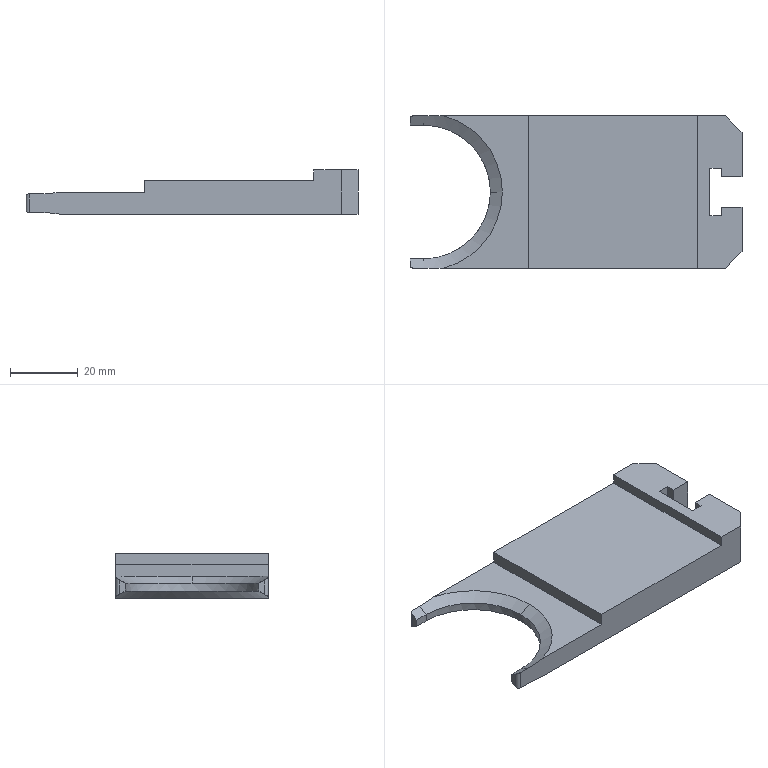Part | SolidWorks | features Chamfer 5, ICE 4, Fillet 2, Cavity 1, Cut 1, Extrusion 1 | 1 solid | 33 faces | box 98 x 45 x 13 mm | volume 33070 mm3 | plane 27 | cone 3 | cylinder 3 | commonest cylinder face diameters 2 x2 39.5 x1
STEP:
#1=CARTESIAN_POINT('',(23.75,0.,-5.62));
#2=VERTEX_POINT('',#1);
#3=CARTESIAN_POINT('',(4.,19.75,-5.62));
#4=VERTEX_POINT('',#3);
#5=CARTESIAN_POINT('',(4.,0.,-5.62));
#6=DIRECTION('',(0.,0.,1.));
#7=DIRECTION('',(-1.,0.,0.));
#8=AXIS2_PLACEMENT_3D('',#5,#6,#7);
#9=CIRCLE('',#8,19.75);
#10=EDGE_CURVE('',#2,#4,#9,.T.);
#11=ORIENTED_EDGE('',*,*,#10,.F.);
#12=CARTESIAN_POINT('',(27.25,0.,-3.6));
#13=VERTEX_POINT('',#12);
#14=CARTESIAN_POINT('',(23.75,0.,-5.62));
#15=DIRECTION('',(0.8661,0.,0.4999));
#16=VECTOR('',#15,1000.);
#17=LINE('',#14,#16);
#18=EDGE_CURVE('',#2,#13,#17,.T.);
#19=ORIENTED_EDGE('',*,*,#18,.T.);
#20=CARTESIAN_POINT('',(9.858,22.5,-3.6));
#21=VERTEX_POINT('',#20);
#22=CARTESIAN_POINT('',(4.,0.,-3.6));
#23=DIRECTION('',(0.,0.,-1.));
#24=DIRECTION('',(-1.,0.,0.));
#25=AXIS2_PLACEMENT_3D('',#22,#23,#24);
#26=CIRCLE('',#25,23.25);
#27=EDGE_CURVE('',#21,#13,#26,.T.);
#28=ORIENTED_EDGE('',*,*,#27,.F.);
#29=CARTESIAN_POINT('',(4.,22.5,-4.033));
#30=VERTEX_POINT('',#29);
#31=CARTESIAN_POINT('',(4.,22.5,-4.033));
#32=CARTESIAN_POINT('',(5.951,22.5,-4.033));
#33=CARTESIAN_POINT('',(7.904,22.5,-3.884));
#34=CARTESIAN_POINT('',(9.858,22.5,-3.6));
#35=B_SPLINE_CURVE_WITH_KNOTS('',3,(#31,#32,#33,#34),.UNSPECIFIED.,.F.,.F.,(4,4),(0.006759,0.01261),.UNSPECIFIED.);
#36=EDGE_CURVE('',#30,#21,#35,.T.);
#37=ORIENTED_EDGE('',*,*,#36,.F.);
#38=CARTESIAN_POINT('',(4.,23.25,-3.6));
#39=DIRECTION('',(0.,-0.8661,-0.4999));
#40=VECTOR('',#39,1000.);
#41=LINE('',#38,#40);
#42=EDGE_CURVE('',#30,#4,#41,.T.);
#43=ORIENTED_EDGE('',*,*,#42,.T.);
#44=EDGE_LOOP('',(#11,#19,#28,#37,#43));
#45=FACE_OUTER_BOUND('',#44,.T.);
#46=CARTESIAN_POINT('',(4.,0.,-5.62));
#47=DIRECTION('',(0.,0.,1.));
#48=DIRECTION('',(1.,0.,0.));
#49=AXIS2_PLACEMENT_3D('',#46,#47,#48);
#50=CONICAL_SURFACE('',#49,19.75,1.047);
#51=ADVANCED_FACE('',(#45),#50,.F.);
#52=CARTESIAN_POINT('',(0.,-21.5,-8.99));
#53=VERTEX_POINT('',#52);
#54=CARTESIAN_POINT('',(0.,-21.5,-4.61));
#55=VERTEX_POINT('',#54);
#56=CARTESIAN_POINT('',(0.,-21.5,-10.));
#57=DIRECTION('',(0.,0.,1.));
#58=VECTOR('',#57,1000.);
#59=LINE('',#56,#58);
#60=EDGE_CURVE('',#53,#55,#59,.T.);
#61=ORIENTED_EDGE('',*,*,#60,.T.);
#62=CARTESIAN_POINT('',(0.,-19.75,-5.62));
#63=VERTEX_POINT('',#62);
#64=CARTESIAN_POINT('',(0.,-19.75,-5.62));
#65=DIRECTION('',(0.,0.8661,-0.4999));
#66=VECTOR('',#65,1000.);
#67=LINE('',#64,#66);
#68=EDGE_CURVE('',#55,#63,#67,.T.);
#69=ORIENTED_EDGE('',*,*,#68,.T.);
#70=CARTESIAN_POINT('',(0.,-19.75,-7.98));
#71=VERTEX_POINT('',#70);
#72=CARTESIAN_POINT('',(0.,-19.75,3.001));
#73=DIRECTION('',(0.,0.,1.));
#74=VECTOR('',#73,1000.);
#75=LINE('',#72,#74);
#76=EDGE_CURVE('',#71,#63,#75,.T.);
#77=ORIENTED_EDGE('',*,*,#76,.F.);
#78=CARTESIAN_POINT('',(0.,-19.75,-7.98));
#79=DIRECTION('',(0.,-0.8661,-0.4999));
#80=VECTOR('',#79,1000.);
#81=LINE('',#78,#80);
#82=EDGE_CURVE('',#71,#53,#81,.T.);
#83=ORIENTED_EDGE('',*,*,#82,.T.);
#84=EDGE_LOOP('',(#61,#69,#77,#83));
#85=FACE_OUTER_BOUND('',#84,.T.);
#86=CARTESIAN_POINT('',(0.,22.5,-10.));
#87=DIRECTION('',(1.,0.,0.));
#88=DIRECTION('',(0.,0.,-1.));
#89=AXIS2_PLACEMENT_3D('',#86,#87,#88);
#90=PLANE('',#89);
#91=ADVANCED_FACE('',(#85),#90,.F.);
#92=CARTESIAN_POINT('',(98.,17.5,3.));
#93=VERTEX_POINT('',#92);
#94=CARTESIAN_POINT('',(98.,4.5,3.));
#95=VERTEX_POINT('',#94);
#96=CARTESIAN_POINT('',(98.,22.5,3.));
#97=DIRECTION('',(0.,-1.,0.));
#98=VECTOR('',#97,1000.);
#99=LINE('',#96,#98);
#100=EDGE_CURVE('',#93,#95,#99,.T.);
#101=ORIENTED_EDGE('',*,*,#100,.T.);
#102=CARTESIAN_POINT('',(98.,4.5,-10.));
#103=VERTEX_POINT('',#102);
#104=CARTESIAN_POINT('',(98.,4.5,3.001));
#105=DIRECTION('',(0.,0.,-1.));
#106=VECTOR('',#105,1000.);
#107=LINE('',#104,#106);
#108=EDGE_CURVE('',#95,#103,#107,.T.);
#109=ORIENTED_EDGE('',*,*,#108,.T.);
#110=CARTESIAN_POINT('',(98.,17.5,-10.));
#111=VERTEX_POINT('',#110);
#112=CARTESIAN_POINT('',(98.,22.5,-10.));
#113=DIRECTION('',(0.,-1.,0.));
#114=VECTOR('',#113,1000.);
#115=LINE('',#112,#114);
#116=EDGE_CURVE('',#111,#103,#115,.T.);
#117=ORIENTED_EDGE('',*,*,#116,.F.);
#118=CARTESIAN_POINT('',(98.,17.5,3.));
#119=DIRECTION('',(0.,0.,1.));
#120=VECTOR('',#119,1000.);
#121=LINE('',#118,#120);
#122=EDGE_CURVE('',#111,#93,#121,.T.);
#123=ORIENTED_EDGE('',*,*,#122,.T.);
#124=EDGE_LOOP('',(#101,#109,#117,#123));
#125=FACE_OUTER_BOUND('',#124,.T.);
#126=CARTESIAN_POINT('',(98.,22.5,3.));
#127=DIRECTION('',(-1.,0.,0.));
#128=DIRECTION('',(0.,0.,1.));
#129=AXIS2_PLACEMENT_3D('',#126,#127,#128);
#130=PLANE('',#129);
#131=ADVANCED_FACE('',(#125),#130,.F.);
#132=CARTESIAN_POINT('',(0.,19.75,-5.62));
#133=VERTEX_POINT('',#132);
#134=CARTESIAN_POINT('',(0.,19.75,-7.98));
#135=VERTEX_POINT('',#134);
#136=CARTESIAN_POINT('',(0.,19.75,3.001));
#137=DIRECTION('',(0.,0.,-1.));
#138=VECTOR('',#137,1000.);
#139=LINE('',#136,#138);
#140=EDGE_CURVE('',#133,#135,#139,.T.);
#141=ORIENTED_EDGE('',*,*,#140,.F.);
#142=CARTESIAN_POINT('',(0.,21.5,-4.61));
#143=VERTEX_POINT('',#142);
#144=CARTESIAN_POINT('',(0.,19.75,-5.62));
#145=DIRECTION('',(0.,0.8661,0.4999));
#146=VECTOR('',#145,1000.);
#147=LINE('',#144,#146);
#148=EDGE_CURVE('',#133,#143,#147,.T.);
#149=ORIENTED_EDGE('',*,*,#148,.T.);
#150=CARTESIAN_POINT('',(0.,21.5,-8.99));
#151=VERTEX_POINT('',#150);
#152=CARTESIAN_POINT('',(0.,21.5,-10.));
#153=DIRECTION('',(0.,0.,-1.));
#154=VECTOR('',#153,1000.);
#155=LINE('',#152,#154);
#156=EDGE_CURVE('',#143,#151,#155,.T.);
#157=ORIENTED_EDGE('',*,*,#156,.T.);
#158=CARTESIAN_POINT('',(0.,19.75,-7.98));
#159=DIRECTION('',(0.,-0.8661,0.4999));
#160=VECTOR('',#159,1000.);
#161=LINE('',#158,#160);
#162=EDGE_CURVE('',#151,#135,#161,.T.);
#163=ORIENTED_EDGE('',*,*,#162,.T.);
#164=EDGE_LOOP('',(#141,#149,#157,#163));
#165=FACE_OUTER_BOUND('',#164,.T.);
#166=CARTESIAN_POINT('',(0.,22.5,-10.));
#167=DIRECTION('',(1.,0.,0.));
#168=DIRECTION('',(0.,0.,-1.));
#169=AXIS2_PLACEMENT_3D('',#166,#167,#168);
#170=PLANE('',#169);
#171=ADVANCED_FACE('',(#165),#170,.F.);
#172=CARTESIAN_POINT('',(35.,22.5,0.));
#173=VERTEX_POINT('',#172);
#174=CARTESIAN_POINT('',(85.,22.5,0.));
#175=VERTEX_POINT('',#174);
#176=CARTESIAN_POINT('',(0.,22.5,0.));
#177=DIRECTION('',(1.,0.,0.));
#178=VECTOR('',#177,1000.);
#179=LINE('',#176,#178);
#180=EDGE_CURVE('',#173,#175,#179,.T.);
#181=ORIENTED_EDGE('',*,*,#180,.F.);
#182=CARTESIAN_POINT('',(35.,-22.5,0.));
#183=VERTEX_POINT('',#182);
#184=CARTESIAN_POINT('',(35.,22.5,0.));
#185=DIRECTION('',(0.,-1.,0.));
#186=VECTOR('',#185,1000.);
#187=LINE('',#184,#186);
#188=EDGE_CURVE('',#173,#183,#187,.T.);
#189=ORIENTED_EDGE('',*,*,#188,.T.);
#190=CARTESIAN_POINT('',(85.,-22.5,0.));
#191=VERTEX_POINT('',#190);
#192=CARTESIAN_POINT('',(0.,-22.5,0.));
#193=DIRECTION('',(1.,0.,0.));
#194=VECTOR('',#193,1000.);
#195=LINE('',#192,#194);
#196=EDGE_CURVE('',#183,#191,#195,.T.);
#197=ORIENTED_EDGE('',*,*,#196,.T.);
#198=CARTESIAN_POINT('',(85.,22.5,0.));
#199=DIRECTION('',(0.,-1.,0.));
#200=VECTOR('',#199,1000.);
#201=LINE('',#198,#200);
#202=EDGE_CURVE('',#175,#191,#201,.T.);
#203=ORIENTED_EDGE('',*,*,#202,.F.);
#204=EDGE_LOOP('',(#181,#189,#197,#203));
#205=FACE_OUTER_BOUND('',#204,.T.);
#206=CARTESIAN_POINT('',(0.,22.5,0.));
#207=DIRECTION('',(0.,0.,-1.));
#208=DIRECTION('',(-1.,0.,0.));
#209=AXIS2_PLACEMENT_3D('',#206,#207,#208);
#210=PLANE('',#209);
#211=ADVANCED_FACE('',(#205),#210,.F.);
#212=CARTESIAN_POINT('',(85.,-22.5,3.));
#213=VERTEX_POINT('',#212);
#214=CARTESIAN_POINT('',(85.,-22.5,0.));
#215=DIRECTION('',(0.,0.,1.));
#216=VECTOR('',#215,1000.);
#217=LINE('',#214,#216);
#218=EDGE_CURVE('',#191,#213,#217,.T.);
#219=ORIENTED_EDGE('',*,*,#218,.T.);
#220=CARTESIAN_POINT('',(85.,22.5,3.));
#221=VERTEX_POINT('',#220);
#222=CARTESIAN_POINT('',(85.,22.5,3.));
#223=DIRECTION('',(0.,-1.,0.));
#224=VECTOR('',#223,1000.);
#225=LINE('',#222,#224);
#226=EDGE_CURVE('',#221,#213,#225,.T.);
#227=ORIENTED_EDGE('',*,*,#226,.F.);
#228=CARTESIAN_POINT('',(85.,22.5,0.));
#229=DIRECTION('',(0.,0.,1.));
#230=VECTOR('',#229,1000.);
#231=LINE('',#228,#230);
#232=EDGE_CURVE('',#175,#221,#231,.T.);
#233=ORIENTED_EDGE('',*,*,#232,.F.);
#234=ORIENTED_EDGE('',*,*,#202,.T.);
#235=EDGE_LOOP('',(#219,#227,#233,#234));
#236=FACE_OUTER_BOUND('',#235,.T.);
#237=CARTESIAN_POINT('',(85.,22.5,0.));
#238=DIRECTION('',(1.,0.,0.));
#239=DIRECTION('',(0.,0.,-1.));
#240=AXIS2_PLACEMENT_3D('',#237,#238,#239);
#241=PLANE('',#240);
#242=ADVANCED_FACE('',(#236),#241,.F.);
#243=CARTESIAN_POINT('',(92.,4.5,3.));
#244=VERTEX_POINT('',#243);
#245=CARTESIAN_POINT('',(92.,7.,3.));
#246=VERTEX_POINT('',#245);
#247=CARTESIAN_POINT('',(92.,4.5,3.));
#248=DIRECTION('',(0.,1.,0.));
#249=VECTOR('',#248,1000.);
#250=LINE('',#247,#249);
#251=EDGE_CURVE('',#244,#246,#250,.T.);
#252=ORIENTED_EDGE('',*,*,#251,.F.);
#253=CARTESIAN_POINT('',(98.,4.5,3.));
#254=DIRECTION('',(-1.,0.,0.));
#255=VECTOR('',#254,1000.);
#256=LINE('',#253,#255);
#257=EDGE_CURVE('',#95,#244,#256,.T.);
#258=ORIENTED_EDGE('',*,*,#257,.F.);
#259=ORIENTED_EDGE('',*,*,#100,.F.);
#260=CARTESIAN_POINT('',(93.,22.5,3.));
#261=VERTEX_POINT('',#260);
#262=CARTESIAN_POINT('',(93.,22.5,3.));
#263=DIRECTION('',(-0.7071,0.7071,0.));
#264=VECTOR('',#263,1000.);
#265=LINE('',#262,#264);
#266=EDGE_CURVE('',#93,#261,#265,.T.);
#267=ORIENTED_EDGE('',*,*,#266,.T.);
#268=CARTESIAN_POINT('',(85.,22.5,3.));
#269=DIRECTION('',(1.,0.,0.));
#270=VECTOR('',#269,1000.);
#271=LINE('',#268,#270);
#272=EDGE_CURVE('',#221,#261,#271,.T.);
#273=ORIENTED_EDGE('',*,*,#272,.F.);
#274=ORIENTED_EDGE('',*,*,#226,.T.);
#275=CARTESIAN_POINT('',(93.,-22.5,3.));
#276=VERTEX_POINT('',#275);
#277=CARTESIAN_POINT('',(85.,-22.5,3.));
#278=DIRECTION('',(1.,0.,0.));
#279=VECTOR('',#278,1000.);
#280=LINE('',#277,#279);
#281=EDGE_CURVE('',#213,#276,#280,.T.);
#282=ORIENTED_EDGE('',*,*,#281,.T.);
#283=CARTESIAN_POINT('',(98.,-17.5,3.));
#284=VERTEX_POINT('',#283);
#285=CARTESIAN_POINT('',(98.,-17.5,3.));
#286=DIRECTION('',(0.7071,0.7071,0.));
#287=VECTOR('',#286,1000.);
#288=LINE('',#285,#287);
#289=EDGE_CURVE('',#276,#284,#288,.T.);
#290=ORIENTED_EDGE('',*,*,#289,.T.);
#291=CARTESIAN_POINT('',(98.,-4.5,3.));
#292=VERTEX_POINT('',#291);
#293=CARTESIAN_POINT('',(98.,22.5,3.));
#294=DIRECTION('',(0.,-1.,0.));
#295=VECTOR('',#294,1000.);
#296=LINE('',#293,#295);
#297=EDGE_CURVE('',#292,#284,#296,.T.);
#298=ORIENTED_EDGE('',*,*,#297,.F.);
#299=CARTESIAN_POINT('',(92.,-4.5,3.));
#300=VERTEX_POINT('',#299);
#301=CARTESIAN_POINT('',(92.,-4.5,3.));
#302=DIRECTION('',(1.,0.,0.));
#303=VECTOR('',#302,1000.);
#304=LINE('',#301,#303);
#305=EDGE_CURVE('',#300,#292,#304,.T.);
#306=ORIENTED_EDGE('',*,*,#305,.F.);
#307=CARTESIAN_POINT('',(92.,-7.,3.));
#308=VERTEX_POINT('',#307);
#309=CARTESIAN_POINT('',(92.,-7.,3.));
#310=DIRECTION('',(0.,1.,0.));
#311=VECTOR('',#310,1000.);
#312=LINE('',#309,#311);
#313=EDGE_CURVE('',#308,#300,#312,.T.);
#314=ORIENTED_EDGE('',*,*,#313,.F.);
#315=CARTESIAN_POINT('',(88.5,-7.,3.));
#316=VERTEX_POINT('',#315);
#317=CARTESIAN_POINT('',(88.5,-7.,3.));
#318=DIRECTION('',(1.,0.,0.));
#319=VECTOR('',#318,1000.);
#320=LINE('',#317,#319);
#321=EDGE_CURVE('',#316,#308,#320,.T.);
#322=ORIENTED_EDGE('',*,*,#321,.F.);
#323=CARTESIAN_POINT('',(88.5,7.,3.));
#324=VERTEX_POINT('',#323);
#325=CARTESIAN_POINT('',(88.5,7.,3.));
#326=DIRECTION('',(0.,-1.,0.));
#327=VECTOR('',#326,1000.);
#328=LINE('',#325,#327);
#329=EDGE_CURVE('',#324,#316,#328,.T.);
#330=ORIENTED_EDGE('',*,*,#329,.F.);
#331=CARTESIAN_POINT('',(92.,7.,3.));
#332=DIRECTION('',(-1.,0.,0.));
#333=VECTOR('',#332,1000.);
#334=LINE('',#331,#333);
#335=EDGE_CURVE('',#246,#324,#334,.T.);
#336=ORIENTED_EDGE('',*,*,#335,.F.);
#337=EDGE_LOOP('',(#252,#258,#259,#267,#273,#274,#282,#290,#298,#306,#314,#322,#330,#336));
#338=FACE_OUTER_BOUND('',#337,.T.);
#339=CARTESIAN_POINT('',(85.,22.5,3.));
#340=DIRECTION('',(0.,0.,-1.));
#341=DIRECTION('',(-1.,0.,0.));
#342=AXIS2_PLACEMENT_3D('',#339,#340,#341);
#343=PLANE('',#342);
#344=ADVANCED_FACE('',(#338),#343,.F.);
#345=CARTESIAN_POINT('',(98.,-4.5,-10.));
#346=VERTEX_POINT('',#345);
#347=CARTESIAN_POINT('',(98.,-17.5,-10.));
#348=VERTEX_POINT('',#347);
#349=CARTESIAN_POINT('',(98.,22.5,-10.));
#350=DIRECTION('',(0.,-1.,0.));
#351=VECTOR('',#350,1000.);
#352=LINE('',#349,#351);
#353=EDGE_CURVE('',#346,#348,#352,.T.);
#354=ORIENTED_EDGE('',*,*,#353,.F.);
#355=CARTESIAN_POINT('',(98.,-4.5,3.001));
#356=DIRECTION('',(0.,0.,-1.));
#357=VECTOR('',#356,1000.);
#358=LINE('',#355,#357);
#359=EDGE_CURVE('',#292,#346,#358,.T.);
#360=ORIENTED_EDGE('',*,*,#359,.F.);
#361=ORIENTED_EDGE('',*,*,#297,.T.);
#362=CARTESIAN_POINT('',(98.,-17.5,3.));
#363=DIRECTION('',(0.,0.,-1.));
#364=VECTOR('',#363,1000.);
#365=LINE('',#362,#364);
#366=EDGE_CURVE('',#284,#348,#365,.T.);
#367=ORIENTED_EDGE('',*,*,#366,.T.);
#368=EDGE_LOOP('',(#354,#360,#361,#367));
#369=FACE_OUTER_BOUND('',#368,.T.);
#370=CARTESIAN_POINT('',(98.,22.5,3.));
#371=DIRECTION('',(-1.,0.,0.));
#372=DIRECTION('',(0.,0.,1.));
#373=AXIS2_PLACEMENT_3D('',#370,#371,#372);
#374=PLANE('',#373);
#375=ADVANCED_FACE('',(#369),#374,.F.);
#376=CARTESIAN_POINT('',(93.,-22.5,-10.));
#377=VERTEX_POINT('',#376);
#378=CARTESIAN_POINT('',(9.858,-22.5,-10.));
#379=VERTEX_POINT('',#378);
#380=CARTESIAN_POINT('',(98.,-22.5,-10.));
#381=DIRECTION('',(-1.,0.,0.));
#382=VECTOR('',#381,1000.);
#383=LINE('',#380,#382);
#384=EDGE_CURVE('',#377,#379,#383,.T.);
#385=ORIENTED_EDGE('',*,*,#384,.T.);
#386=CARTESIAN_POINT('',(9.858,22.5,-10.));
#387=VERTEX_POINT('',#386);
#388=CARTESIAN_POINT('',(4.,0.,-10.));
#389=DIRECTION('',(0.,0.,1.));
#390=DIRECTION('',(1.,0.,0.));
#391=AXIS2_PLACEMENT_3D('',#388,#389,#390);
#392=CIRCLE('',#391,23.25);
#393=EDGE_CURVE('',#379,#387,#392,.T.);
#394=ORIENTED_EDGE('',*,*,#393,.T.);
#395=CARTESIAN_POINT('',(93.,22.5,-10.));
#396=VERTEX_POINT('',#395);
#397=CARTESIAN_POINT('',(98.,22.5,-10.));
#398=DIRECTION('',(-1.,0.,0.));
#399=VECTOR('',#398,1000.);
#400=LINE('',#397,#399);
#401=EDGE_CURVE('',#396,#387,#400,.T.);
#402=ORIENTED_EDGE('',*,*,#401,.F.);
#403=CARTESIAN_POINT('',(93.,22.5,-10.));
#404=DIRECTION('',(0.7071,-0.7071,0.));
#405=VECTOR('',#404,1000.);
#406=LINE('',#403,#405);
#407=EDGE_CURVE('',#396,#111,#406,.T.);
#408=ORIENTED_EDGE('',*,*,#407,.T.);
#409=ORIENTED_EDGE('',*,*,#116,.T.);
#410=CARTESIAN_POINT('',(92.,4.5,-10.));
#411=VERTEX_POINT('',#410);
#412=CARTESIAN_POINT('',(98.,4.5,-10.));
#413=DIRECTION('',(1.,0.,0.));
#414=VECTOR('',#413,1000.);
#415=LINE('',#412,#414);
#416=EDGE_CURVE('',#411,#103,#415,.T.);
#417=ORIENTED_EDGE('',*,*,#416,.F.);
#418=CARTESIAN_POINT('',(92.,7.,-10.));
#419=VERTEX_POINT('',#418);
#420=CARTESIAN_POINT('',(92.,4.5,-10.));
#421=DIRECTION('',(0.,-1.,0.));
#422=VECTOR('',#421,1000.);
#423=LINE('',#420,#422);
#424=EDGE_CURVE('',#419,#411,#423,.T.);
#425=ORIENTED_EDGE('',*,*,#424,.F.);
#426=CARTESIAN_POINT('',(88.5,7.,-10.));
#427=VERTEX_POINT('',#426);
#428=CARTESIAN_POINT('',(92.,7.,-10.));
#429=DIRECTION('',(1.,0.,0.));
#430=VECTOR('',#429,1000.);
#431=LINE('',#428,#430);
#432=EDGE_CURVE('',#427,#419,#431,.T.);
#433=ORIENTED_EDGE('',*,*,#432,.F.);
#434=CARTESIAN_POINT('',(88.5,-7.,-10.));
#435=VERTEX_POINT('',#434);
#436=CARTESIAN_POINT('',(88.5,7.,-10.));
#437=DIRECTION('',(0.,1.,0.));
#438=VECTOR('',#437,1000.);
#439=LINE('',#436,#438);
#440=EDGE_CURVE('',#435,#427,#439,.T.);
#441=ORIENTED_EDGE('',*,*,#440,.F.);
#442=CARTESIAN_POINT('',(92.,-7.,-10.));
#443=VERTEX_POINT('',#442);
#444=CARTESIAN_POINT('',(88.5,-7.,-10.));
#445=DIRECTION('',(-1.,0.,0.));
#446=VECTOR('',#445,1000.);
#447=LINE('',#444,#446);
#448=EDGE_CURVE('',#443,#435,#447,.T.);
#449=ORIENTED_EDGE('',*,*,#448,.F.);
#450=CARTESIAN_POINT('',(92.,-4.5,-10.));
#451=VERTEX_POINT('',#450);
#452=CARTESIAN_POINT('',(92.,-7.,-10.));
#453=DIRECTION('',(0.,-1.,0.));
#454=VECTOR('',#453,1000.);
#455=LINE('',#452,#454);
#456=EDGE_CURVE('',#451,#443,#455,.T.);
#457=ORIENTED_EDGE('',*,*,#456,.F.);
#458=CARTESIAN_POINT('',(92.,-4.5,-10.));
#459=DIRECTION('',(-1.,0.,0.));
#460=VECTOR('',#459,1000.);
#461=LINE('',#458,#460);
#462=EDGE_CURVE('',#346,#451,#461,.T.);
#463=ORIENTED_EDGE('',*,*,#462,.F.);
#464=ORIENTED_EDGE('',*,*,#353,.T.);
#465=CARTESIAN_POINT('',(98.,-17.5,-10.));
#466=DIRECTION('',(-0.7071,-0.7071,0.));
#467=VECTOR('',#466,1000.);
#468=LINE('',#465,#467);
#469=EDGE_CURVE('',#348,#377,#468,.T.);
#470=ORIENTED_EDGE('',*,*,#469,.T.);
#471=EDGE_LOOP('',(#385,#394,#402,#408,#409,#417,#425,#433,#441,#449,#457,#463,#464,#470));
#472=FACE_OUTER_BOUND('',#471,.T.);
#473=CARTESIAN_POINT('',(98.,22.5,-10.));
#474=DIRECTION('',(0.,0.,1.));
#475=DIRECTION('',(1.,0.,0.));
#476=AXIS2_PLACEMENT_3D('',#473,#474,#475);
#477=PLANE('',#476);
#478=ADVANCED_FACE('',(#472),#477,.F.);
#479=CARTESIAN_POINT('',(1.,22.5,-9.567));
#480=VERTEX_POINT('',#479);
#481=CARTESIAN_POINT('',(1.,22.5,-4.033));
#482=VERTEX_POINT('',#481);
#483=CARTESIAN_POINT('',(1.,22.5,0.));
#484=DIRECTION('',(0.,0.,1.));
#485=VECTOR('',#484,1000.);
#486=LINE('',#483,#485);
#487=EDGE_CURVE('',#480,#482,#486,.T.);
#488=ORIENTED_EDGE('',*,*,#487,.T.);
#489=CARTESIAN_POINT('',(0.,22.5,-4.033));
#490=DIRECTION('',(1.,0.,0.));
#491=VECTOR('',#490,1000.);
#492=LINE('',#489,#491);
#493=EDGE_CURVE('',#482,#30,#492,.T.);
#494=ORIENTED_EDGE('',*,*,#493,.T.);
#495=ORIENTED_EDGE('',*,*,#36,.T.);
#496=CARTESIAN_POINT('',(35.,22.5,-3.6));
#497=VERTEX_POINT('',#496);
#498=CARTESIAN_POINT('',(0.,22.5,-3.6));
#499=DIRECTION('',(1.,0.,0.));
#500=VECTOR('',#499,1000.);
#501=LINE('',#498,#500);
#502=EDGE_CURVE('',#21,#497,#501,.T.);
#503=ORIENTED_EDGE('',*,*,#502,.T.);
#504=CARTESIAN_POINT('',(35.,22.5,0.));
#505=DIRECTION('',(0.,0.,1.));
#506=VECTOR('',#505,1000.);
#507=LINE('',#504,#506);
#508=EDGE_CURVE('',#497,#173,#507,.T.);
#509=ORIENTED_EDGE('',*,*,#508,.T.);
#510=ORIENTED_EDGE('',*,*,#180,.T.);
#511=ORIENTED_EDGE('',*,*,#232,.T.);
#512=ORIENTED_EDGE('',*,*,#272,.T.);
#513=CARTESIAN_POINT('',(93.,22.5,-10.));
#514=DIRECTION('',(0.,0.,-1.));
#515=VECTOR('',#514,1000.);
#516=LINE('',#513,#515);
#517=EDGE_CURVE('',#261,#396,#516,.T.);
#518=ORIENTED_EDGE('',*,*,#517,.T.);
#519=ORIENTED_EDGE('',*,*,#401,.T.);
#520=CARTESIAN_POINT('',(4.,22.5,-9.567));
#521=VERTEX_POINT('',#520);
#522=CARTESIAN_POINT('',(9.858,22.5,-10.));
#523=CARTESIAN_POINT('',(7.904,22.5,-9.716));
#524=CARTESIAN_POINT('',(5.951,22.5,-9.567));
#525=CARTESIAN_POINT('',(4.,22.5,-9.567));
#526=B_SPLINE_CURVE_WITH_KNOTS('',3,(#522,#523,#524,#525),.UNSPECIFIED.,.F.,.F.,(4,4),(0.,0.005853),.UNSPECIFIED.);
#527=EDGE_CURVE('',#387,#521,#526,.T.);
#528=ORIENTED_EDGE('',*,*,#527,.T.);
#529=CARTESIAN_POINT('',(0.,22.5,-9.567));
#530=DIRECTION('',(-1.,0.,0.));
#531=VECTOR('',#530,1000.);
#532=LINE('',#529,#531);
#533=EDGE_CURVE('',#521,#480,#532,.T.);
#534=ORIENTED_EDGE('',*,*,#533,.T.);
#535=EDGE_LOOP('',(#488,#494,#495,#503,#509,#510,#511,#512,#518,#519,#528,#534));
#536=FACE_OUTER_BOUND('',#535,.T.);
#537=CARTESIAN_POINT('',(0.,22.5,0.));
#538=DIRECTION('',(0.,1.,0.));
#539=DIRECTION('',(0.,0.,1.));
#540=AXIS2_PLACEMENT_3D('',#537,#538,#539);
#541=PLANE('',#540);
#542=ADVANCED_FACE('',(#536),#541,.T.);
#543=CARTESIAN_POINT('',(9.858,-22.5,-3.6));
#544=VERTEX_POINT('',#543);
#545=CARTESIAN_POINT('',(4.,-22.5,-4.033));
#546=VERTEX_POINT('',#545);
#547=CARTESIAN_POINT('',(9.858,-22.5,-3.6));
#548=CARTESIAN_POINT('',(7.904,-22.5,-3.884));
#549=CARTESIAN_POINT('',(5.951,-22.5,-4.033));
#550=CARTESIAN_POINT('',(4.,-22.5,-4.033));
#551=B_SPLINE_CURVE_WITH_KNOTS('',3,(#547,#548,#549,#550),.UNSPECIFIED.,.F.,.F.,(4,4),(0.,0.005853),.UNSPECIFIED.);
#552=EDGE_CURVE('',#544,#546,#551,.T.);
#553=ORIENTED_EDGE('',*,*,#552,.T.);
#554=CARTESIAN_POINT('',(1.,-22.5,-4.033));
#555=VERTEX_POINT('',#554);
#556=CARTESIAN_POINT('',(-4.,-22.5,-4.033));
#557=DIRECTION('',(-1.,0.,0.));
#558=VECTOR('',#557,1000.);
#559=LINE('',#556,#558);
#560=EDGE_CURVE('',#546,#555,#559,.T.);
#561=ORIENTED_EDGE('',*,*,#560,.T.);
#562=CARTESIAN_POINT('',(1.,-22.5,-9.567));
#563=VERTEX_POINT('',#562);
#564=CARTESIAN_POINT('',(1.,-22.5,0.));
#565=DIRECTION('',(0.,0.,-1.));
#566=VECTOR('',#565,1000.);
#567=LINE('',#564,#566);
#568=EDGE_CURVE('',#555,#563,#567,.T.);
#569=ORIENTED_EDGE('',*,*,#568,.T.);
#570=CARTESIAN_POINT('',(4.,-22.5,-9.567));
#571=VERTEX_POINT('',#570);
#572=CARTESIAN_POINT('',(-4.,-22.5,-9.567));
#573=DIRECTION('',(1.,0.,0.));
#574=VECTOR('',#573,1000.);
#575=LINE('',#572,#574);
#576=EDGE_CURVE('',#563,#571,#575,.T.);
#577=ORIENTED_EDGE('',*,*,#576,.T.);
#578=CARTESIAN_POINT('',(4.,-22.5,-9.567));
#579=CARTESIAN_POINT('',(5.951,-22.5,-9.567));
#580=CARTESIAN_POINT('',(7.904,-22.5,-9.716));
#581=CARTESIAN_POINT('',(9.858,-22.5,-10.));
#582=B_SPLINE_CURVE_WITH_KNOTS('',3,(#578,#579,#580,#581),.UNSPECIFIED.,.F.,.F.,(4,4),(0.006759,0.01261),.UNSPECIFIED.);
#583=EDGE_CURVE('',#571,#379,#582,.T.);
#584=ORIENTED_EDGE('',*,*,#583,.T.);
#585=ORIENTED_EDGE('',*,*,#384,.F.);
#586=CARTESIAN_POINT('',(93.,-22.5,0.));
#587=DIRECTION('',(0.,0.,1.));
#588=VECTOR('',#587,1000.);
#589=LINE('',#586,#588);
#590=EDGE_CURVE('',#377,#276,#589,.T.);
#591=ORIENTED_EDGE('',*,*,#590,.T.);
#592=ORIENTED_EDGE('',*,*,#281,.F.);
#593=ORIENTED_EDGE('',*,*,#218,.F.);
#594=ORIENTED_EDGE('',*,*,#196,.F.);
#595=CARTESIAN_POINT('',(35.,-22.5,-3.6));
#596=VERTEX_POINT('',#595);
#597=CARTESIAN_POINT('',(35.,-22.5,0.));
#598=DIRECTION('',(0.,0.,1.));
#599=VECTOR('',#598,1000.);
#600=LINE('',#597,#599);
#601=EDGE_CURVE('',#596,#183,#600,.T.);
#602=ORIENTED_EDGE('',*,*,#601,.F.);
#603=CARTESIAN_POINT('',(0.,-22.5,-3.6));
#604=DIRECTION('',(1.,0.,0.));
#605=VECTOR('',#604,1000.);
#606=LINE('',#603,#605);
#607=EDGE_CURVE('',#544,#596,#606,.T.);
#608=ORIENTED_EDGE('',*,*,#607,.F.);
#609=EDGE_LOOP('',(#553,#561,#569,#577,#584,#585,#591,#592,#593,#594,#602,#608));
#610=FACE_OUTER_BOUND('',#609,.T.);
#611=CARTESIAN_POINT('',(0.,-22.5,0.));
#612=DIRECTION('',(0.,1.,0.));
#613=DIRECTION('',(0.,0.,1.));
#614=AXIS2_PLACEMENT_3D('',#611,#612,#613);
#615=PLANE('',#614);
#616=ADVANCED_FACE('',(#610),#615,.F.);
#617=ORIENTED_EDGE('',*,*,#289,.F.);
#618=ORIENTED_EDGE('',*,*,#590,.F.);
#619=ORIENTED_EDGE('',*,*,#469,.F.);
#620=ORIENTED_EDGE('',*,*,#366,.F.);
#621=EDGE_LOOP('',(#617,#618,#619,#620));
#622=FACE_OUTER_BOUND('',#621,.T.);
#623=CARTESIAN_POINT('',(98.,-17.5,3.));
#624=DIRECTION('',(-0.7071,0.7071,0.));
#625=DIRECTION('',(0.,0.,-1.));
#626=AXIS2_PLACEMENT_3D('',#623,#624,#625);
#627=PLANE('',#626);
#628=ADVANCED_FACE('',(#622),#627,.F.);
#629=ORIENTED_EDGE('',*,*,#266,.F.);
#630=ORIENTED_EDGE('',*,*,#122,.F.);
#631=ORIENTED_EDGE('',*,*,#407,.F.);
#632=ORIENTED_EDGE('',*,*,#517,.F.);
#633=EDGE_LOOP('',(#629,#630,#631,#632));
#634=FACE_OUTER_BOUND('',#633,.T.);
#635=CARTESIAN_POINT('',(93.,22.5,0.));
#636=DIRECTION('',(0.7071,0.7071,0.));
#637=DIRECTION('',(0.,0.,1.));
#638=AXIS2_PLACEMENT_3D('',#635,#636,#637);
#639=PLANE('',#638);
#640=ADVANCED_FACE('',(#634),#639,.T.);
#641=ORIENTED_EDGE('',*,*,#568,.F.);
#642=CARTESIAN_POINT('',(1.,-22.5,-4.033));
#643=CARTESIAN_POINT('',(0.4142,-22.5,-4.033));
#644=CARTESIAN_POINT('',(0.,-22.086,-4.272));
#645=CARTESIAN_POINT('',(0.,-21.5,-4.61));
#646=(BOUNDED_CURVE()B_SPLINE_CURVE(3,(#642,#643,#644,#645),.UNSPECIFIED.,.F.,.T.)B_SPLINE_CURVE_WITH_KNOTS((4,4),(0.,1.571),.UNSPECIFIED.)CURVE()GEOMETRIC_REPRESENTATION_ITEM()RATIONAL_B_SPLINE_CURVE((1.,0.8047,0.8047,1.))REPRESENTATION_ITEM(''));
#647=EDGE_CURVE('',#555,#55,#646,.T.);
#648=ORIENTED_EDGE('',*,*,#647,.T.);
#649=ORIENTED_EDGE('',*,*,#60,.F.);
#650=CARTESIAN_POINT('',(0.,-21.5,-8.99));
#651=CARTESIAN_POINT('',(0.,-22.086,-9.328));
#652=CARTESIAN_POINT('',(0.4142,-22.5,-9.567));
#653=CARTESIAN_POINT('',(1.,-22.5,-9.567));
#654=(BOUNDED_CURVE()B_SPLINE_CURVE(3,(#650,#651,#652,#653),.UNSPECIFIED.,.F.,.T.)B_SPLINE_CURVE_WITH_KNOTS((4,4),(1.571,3.142),.UNSPECIFIED.)CURVE()GEOMETRIC_REPRESENTATION_ITEM()RATIONAL_B_SPLINE_CURVE((1.,0.8047,0.8047,1.))REPRESENTATION_ITEM(''));
#655=EDGE_CURVE('',#53,#563,#654,.T.);
#656=ORIENTED_EDGE('',*,*,#655,.T.);
#657=EDGE_LOOP('',(#641,#648,#649,#656));
#658=FACE_OUTER_BOUND('',#657,.T.);
#659=CARTESIAN_POINT('',(1.,-21.5,-10.));
#660=DIRECTION('',(0.,0.,1.));
#661=DIRECTION('',(1.,0.,0.));
#662=AXIS2_PLACEMENT_3D('',#659,#660,#661);
#663=CYLINDRICAL_SURFACE('',#662,1.);
#664=ADVANCED_FACE('',(#658),#663,.T.);
#665=ORIENTED_EDGE('',*,*,#156,.F.);
#666=CARTESIAN_POINT('',(0.,21.5,-4.61));
#667=CARTESIAN_POINT('',(0.,22.086,-4.272));
#668=CARTESIAN_POINT('',(0.4142,22.5,-4.033));
#669=CARTESIAN_POINT('',(1.,22.5,-4.033));
#670=(BOUNDED_CURVE()B_SPLINE_CURVE(3,(#666,#667,#668,#669),.UNSPECIFIED.,.F.,.T.)B_SPLINE_CURVE_WITH_KNOTS((4,4),(1.571,3.142),.UNSPECIFIED.)CURVE()GEOMETRIC_REPRESENTATION_ITEM()RATIONAL_B_SPLINE_CURVE((1.,0.8047,0.8047,1.))REPRESENTATION_ITEM(''));
#671=EDGE_CURVE('',#143,#482,#670,.T.);
#672=ORIENTED_EDGE('',*,*,#671,.T.);
#673=ORIENTED_EDGE('',*,*,#487,.F.);
#674=CARTESIAN_POINT('',(1.,22.5,-9.567));
#675=CARTESIAN_POINT('',(0.4142,22.5,-9.567));
#676=CARTESIAN_POINT('',(0.,22.086,-9.328));
#677=CARTESIAN_POINT('',(0.,21.5,-8.99));
#678=(BOUNDED_CURVE()B_SPLINE_CURVE(3,(#674,#675,#676,#677),.UNSPECIFIED.,.F.,.T.)B_SPLINE_CURVE_WITH_KNOTS((4,4),(0.,1.571),.UNSPECIFIED.)CURVE()GEOMETRIC_REPRESENTATION_ITEM()RATIONAL_B_SPLINE_CURVE((1.,0.8047,0.8047,1.))REPRESENTATION_ITEM(''));
#679=EDGE_CURVE('',#480,#151,#678,.T.);
#680=ORIENTED_EDGE('',*,*,#679,.T.);
#681=EDGE_LOOP('',(#665,#672,#673,#680));
#682=FACE_OUTER_BOUND('',#681,.T.);
#683=CARTESIAN_POINT('',(1.,21.5,0.));
#684=DIRECTION('',(0.,0.,-1.));
#685=DIRECTION('',(-1.,0.,0.));
#686=AXIS2_PLACEMENT_3D('',#683,#684,#685);
#687=CYLINDRICAL_SURFACE('',#686,1.);
#688=ADVANCED_FACE('',(#682),#687,.T.);
#689=ORIENTED_EDGE('',*,*,#257,.T.);
#690=CARTESIAN_POINT('',(92.,4.5,3.001));
#691=DIRECTION('',(0.,0.,-1.));
#692=VECTOR('',#691,1000.);
#693=LINE('',#690,#692);
#694=EDGE_CURVE('',#244,#411,#693,.T.);
#695=ORIENTED_EDGE('',*,*,#694,.T.);
#696=ORIENTED_EDGE('',*,*,#416,.T.);
#697=ORIENTED_EDGE('',*,*,#108,.F.);
#698=EDGE_LOOP('',(#689,#695,#696,#697));
#699=FACE_OUTER_BOUND('',#698,.T.);
#700=CARTESIAN_POINT('',(98.,4.5,3.001));
#701=DIRECTION('',(0.,1.,0.));
#702=DIRECTION('',(-1.,0.,0.));
#703=AXIS2_PLACEMENT_3D('',#700,#701,#702);
#704=PLANE('',#703);
#705=ADVANCED_FACE('',(#699),#704,.F.);
#706=ORIENTED_EDGE('',*,*,#251,.T.);
#707=CARTESIAN_POINT('',(92.,7.,3.001));
#708=DIRECTION('',(0.,0.,-1.));
#709=VECTOR('',#708,1000.);
#710=LINE('',#707,#709);
#711=EDGE_CURVE('',#246,#419,#710,.T.);
#712=ORIENTED_EDGE('',*,*,#711,.T.);
#713=ORIENTED_EDGE('',*,*,#424,.T.);
#714=ORIENTED_EDGE('',*,*,#694,.F.);
#715=EDGE_LOOP('',(#706,#712,#713,#714));
#716=FACE_OUTER_BOUND('',#715,.T.);
#717=CARTESIAN_POINT('',(92.,4.5,3.001));
#718=DIRECTION('',(1.,0.,0.));
#719=DIRECTION('',(0.,0.,-1.));
#720=AXIS2_PLACEMENT_3D('',#717,#718,#719);
#721=PLANE('',#720);
#722=ADVANCED_FACE('',(#716),#721,.F.);
#723=ORIENTED_EDGE('',*,*,#335,.T.);
#724=CARTESIAN_POINT('',(88.5,7.,3.001));
#725=DIRECTION('',(0.,0.,-1.));
#726=VECTOR('',#725,1000.);
#727=LINE('',#724,#726);
#728=EDGE_CURVE('',#324,#427,#727,.T.);
#729=ORIENTED_EDGE('',*,*,#728,.T.);
#730=ORIENTED_EDGE('',*,*,#432,.T.);
#731=ORIENTED_EDGE('',*,*,#711,.F.);
#732=EDGE_LOOP('',(#723,#729,#730,#731));
#733=FACE_OUTER_BOUND('',#732,.T.);
#734=CARTESIAN_POINT('',(92.,7.,3.001));
#735=DIRECTION('',(0.,1.,0.));
#736=DIRECTION('',(0.,0.,1.));
#737=AXIS2_PLACEMENT_3D('',#734,#735,#736);
#738=PLANE('',#737);
#739=ADVANCED_FACE('',(#733),#738,.F.);
#740=ORIENTED_EDGE('',*,*,#329,.T.);
#741=CARTESIAN_POINT('',(88.5,-7.,3.001));
#742=DIRECTION('',(0.,0.,-1.));
#743=VECTOR('',#742,1000.);
#744=LINE('',#741,#743);
#745=EDGE_CURVE('',#316,#435,#744,.T.);
#746=ORIENTED_EDGE('',*,*,#745,.T.);
#747=ORIENTED_EDGE('',*,*,#440,.T.);
#748=ORIENTED_EDGE('',*,*,#728,.F.);
#749=EDGE_LOOP('',(#740,#746,#747,#748));
#750=FACE_OUTER_BOUND('',#749,.T.);
#751=CARTESIAN_POINT('',(88.5,7.,3.001));
#752=DIRECTION('',(-1.,0.,0.));
#753=DIRECTION('',(0.,0.,1.));
#754=AXIS2_PLACEMENT_3D('',#751,#752,#753);
#755=PLANE('',#754);
#756=ADVANCED_FACE('',(#750),#755,.F.);
#757=ORIENTED_EDGE('',*,*,#321,.T.);
#758=CARTESIAN_POINT('',(92.,-7.,3.001));
#759=DIRECTION('',(0.,0.,-1.));
#760=VECTOR('',#759,1000.);
#761=LINE('',#758,#760);
#762=EDGE_CURVE('',#308,#443,#761,.T.);
#763=ORIENTED_EDGE('',*,*,#762,.T.);
#764=ORIENTED_EDGE('',*,*,#448,.T.);
#765=ORIENTED_EDGE('',*,*,#745,.F.);
#766=EDGE_LOOP('',(#757,#763,#764,#765));
#767=FACE_OUTER_BOUND('',#766,.T.);
#768=CARTESIAN_POINT('',(88.5,-7.,3.001));
#769=DIRECTION('',(0.,-1.,0.));
#770=DIRECTION('',(1.,0.,0.));
#771=AXIS2_PLACEMENT_3D('',#768,#769,#770);
#772=PLANE('',#771);
#773=ADVANCED_FACE('',(#767),#772,.F.);
#774=ORIENTED_EDGE('',*,*,#313,.T.);
#775=CARTESIAN_POINT('',(92.,-4.5,3.001));
#776=DIRECTION('',(0.,0.,-1.));
#777=VECTOR('',#776,1000.);
#778=LINE('',#775,#777);
#779=EDGE_CURVE('',#300,#451,#778,.T.);
#780=ORIENTED_EDGE('',*,*,#779,.T.);
#781=ORIENTED_EDGE('',*,*,#456,.T.);
#782=ORIENTED_EDGE('',*,*,#762,.F.);
#783=EDGE_LOOP('',(#774,#780,#781,#782));
#784=FACE_OUTER_BOUND('',#783,.T.);
#785=CARTESIAN_POINT('',(92.,-7.,3.001));
#786=DIRECTION('',(1.,0.,0.));
#787=DIRECTION('',(0.,0.,-1.));
#788=AXIS2_PLACEMENT_3D('',#785,#786,#787);
#789=PLANE('',#788);
#790=ADVANCED_FACE('',(#784),#789,.F.);
#791=ORIENTED_EDGE('',*,*,#305,.T.);
#792=ORIENTED_EDGE('',*,*,#359,.T.);
#793=ORIENTED_EDGE('',*,*,#462,.T.);
#794=ORIENTED_EDGE('',*,*,#779,.F.);
#795=EDGE_LOOP('',(#791,#792,#793,#794));
#796=FACE_OUTER_BOUND('',#795,.T.);
#797=CARTESIAN_POINT('',(92.,-4.5,3.001));
#798=DIRECTION('',(0.,-1.,0.));
#799=DIRECTION('',(0.,0.,-1.));
#800=AXIS2_PLACEMENT_3D('',#797,#798,#799);
#801=PLANE('',#800);
#802=ADVANCED_FACE('',(#796),#801,.F.);
#803=ORIENTED_EDGE('',*,*,#76,.T.);
#804=CARTESIAN_POINT('',(4.,-19.75,-5.62));
#805=VERTEX_POINT('',#804);
#806=CARTESIAN_POINT('',(-4.,-19.75,-5.62));
#807=DIRECTION('',(1.,0.,0.));
#808=VECTOR('',#807,1000.);
#809=LINE('',#806,#808);
#810=EDGE_CURVE('',#63,#805,#809,.T.);
#811=ORIENTED_EDGE('',*,*,#810,.T.);
#812=CARTESIAN_POINT('',(4.,-19.75,-7.98));
#813=VERTEX_POINT('',#812);
#814=CARTESIAN_POINT('',(4.,-19.75,3.001));
#815=DIRECTION('',(0.,0.,-1.));
#816=VECTOR('',#815,1000.);
#817=LINE('',#814,#816);
#818=EDGE_CURVE('',#805,#813,#817,.T.);
#819=ORIENTED_EDGE('',*,*,#818,.T.);
#820=CARTESIAN_POINT('',(-4.,-19.75,-7.98));
#821=DIRECTION('',(-1.,0.,0.));
#822=VECTOR('',#821,1000.);
#823=LINE('',#820,#822);
#824=EDGE_CURVE('',#813,#71,#823,.T.);
#825=ORIENTED_EDGE('',*,*,#824,.T.);
#826=EDGE_LOOP('',(#803,#811,#819,#825));
#827=FACE_OUTER_BOUND('',#826,.T.);
#828=CARTESIAN_POINT('',(-4.,-19.75,3.001));
#829=DIRECTION('',(0.,-1.,0.));
#830=DIRECTION('',(1.,0.,0.));
#831=AXIS2_PLACEMENT_3D('',#828,#829,#830);
#832=PLANE('',#831);
#833=ADVANCED_FACE('',(#827),#832,.F.);
#834=ORIENTED_EDGE('',*,*,#818,.F.);
#835=CARTESIAN_POINT('',(4.,0.,-5.62));
#836=DIRECTION('',(0.,0.,1.));
#837=DIRECTION('',(-1.,0.,0.));
#838=AXIS2_PLACEMENT_3D('',#835,#836,#837);
#839=CIRCLE('',#838,19.75);
#840=EDGE_CURVE('',#805,#2,#839,.T.);
#841=ORIENTED_EDGE('',*,*,#840,.T.);
#842=ORIENTED_EDGE('',*,*,#10,.T.);
#843=CARTESIAN_POINT('',(4.,19.75,-7.98));
#844=VERTEX_POINT('',#843);
#845=CARTESIAN_POINT('',(4.,19.75,3.001));
#846=DIRECTION('',(0.,0.,-1.));
#847=VECTOR('',#846,1000.);
#848=LINE('',#845,#847);
#849=EDGE_CURVE('',#4,#844,#848,.T.);
#850=ORIENTED_EDGE('',*,*,#849,.T.);
#851=CARTESIAN_POINT('',(4.,0.,-7.98));
#852=DIRECTION('',(0.,0.,-1.));
#853=DIRECTION('',(1.,0.,0.));
#854=AXIS2_PLACEMENT_3D('',#851,#852,#853);
#855=CIRCLE('',#854,19.75);
#856=EDGE_CURVE('',#844,#813,#855,.T.);
#857=ORIENTED_EDGE('',*,*,#856,.T.);
#858=EDGE_LOOP('',(#834,#841,#842,#850,#857));
#859=FACE_OUTER_BOUND('',#858,.T.);
#860=CARTESIAN_POINT('',(4.,0.,3.001));
#861=DIRECTION('',(0.,0.,-1.));
#862=DIRECTION('',(-1.,0.,0.));
#863=AXIS2_PLACEMENT_3D('',#860,#861,#862);
#864=CYLINDRICAL_SURFACE('',#863,19.75);
#865=ADVANCED_FACE('',(#859),#864,.F.);
#866=ORIENTED_EDGE('',*,*,#849,.F.);
#867=CARTESIAN_POINT('',(-4.,19.75,-5.62));
#868=DIRECTION('',(-1.,0.,0.));
#869=VECTOR('',#868,1000.);
#870=LINE('',#867,#869);
#871=EDGE_CURVE('',#4,#133,#870,.T.);
#872=ORIENTED_EDGE('',*,*,#871,.T.);
#873=ORIENTED_EDGE('',*,*,#140,.T.);
#874=CARTESIAN_POINT('',(-4.,19.75,-7.98));
#875=DIRECTION('',(1.,0.,0.));
#876=VECTOR('',#875,1000.);
#877=LINE('',#874,#876);
#878=EDGE_CURVE('',#135,#844,#877,.T.);
#879=ORIENTED_EDGE('',*,*,#878,.T.);
#880=EDGE_LOOP('',(#866,#872,#873,#879));
#881=FACE_OUTER_BOUND('',#880,.T.);
#882=CARTESIAN_POINT('',(-4.,19.75,3.001));
#883=DIRECTION('',(0.,1.,0.));
#884=DIRECTION('',(-1.,0.,0.));
#885=AXIS2_PLACEMENT_3D('',#882,#883,#884);
#886=PLANE('',#885);
#887=ADVANCED_FACE('',(#881),#886,.F.);
#888=ORIENTED_EDGE('',*,*,#502,.F.);
#889=ORIENTED_EDGE('',*,*,#27,.T.);
#890=CARTESIAN_POINT('',(4.,0.,-3.6));
#891=DIRECTION('',(0.,0.,-1.));
#892=DIRECTION('',(-1.,0.,0.));
#893=AXIS2_PLACEMENT_3D('',#890,#891,#892);
#894=CIRCLE('',#893,23.25);
#895=EDGE_CURVE('',#13,#544,#894,.T.);
#896=ORIENTED_EDGE('',*,*,#895,.T.);
#897=ORIENTED_EDGE('',*,*,#607,.T.);
#898=CARTESIAN_POINT('',(35.,22.5,-3.6));
#899=DIRECTION('',(0.,-1.,0.));
#900=VECTOR('',#899,1000.);
#901=LINE('',#898,#900);
#902=EDGE_CURVE('',#497,#596,#901,.T.);
#903=ORIENTED_EDGE('',*,*,#902,.F.);
#904=EDGE_LOOP('',(#888,#889,#896,#897,#903));
#905=FACE_OUTER_BOUND('',#904,.T.);
#906=CARTESIAN_POINT('',(0.,22.5,-3.6));
#907=DIRECTION('',(0.,0.,-1.));
#908=DIRECTION('',(-1.,0.,0.));
#909=AXIS2_PLACEMENT_3D('',#906,#907,#908);
#910=PLANE('',#909);
#911=ADVANCED_FACE('',(#905),#910,.F.);
#912=ORIENTED_EDGE('',*,*,#601,.T.);
#913=ORIENTED_EDGE('',*,*,#188,.F.);
#914=ORIENTED_EDGE('',*,*,#508,.F.);
#915=ORIENTED_EDGE('',*,*,#902,.T.);
#916=EDGE_LOOP('',(#912,#913,#914,#915));
#917=FACE_OUTER_BOUND('',#916,.T.);
#918=CARTESIAN_POINT('',(35.,22.5,0.));
#919=DIRECTION('',(1.,0.,0.));
#920=DIRECTION('',(0.,0.,-1.));
#921=AXIS2_PLACEMENT_3D('',#918,#919,#920);
#922=PLANE('',#921);
#923=ADVANCED_FACE('',(#917),#922,.F.);
#924=ORIENTED_EDGE('',*,*,#82,.F.);
#925=ORIENTED_EDGE('',*,*,#824,.F.);
#926=CARTESIAN_POINT('',(4.,-23.25,-10.));
#927=DIRECTION('',(0.,0.8661,0.4999));
#928=VECTOR('',#927,1000.);
#929=LINE('',#926,#928);
#930=EDGE_CURVE('',#571,#813,#929,.T.);
#931=ORIENTED_EDGE('',*,*,#930,.F.);
#932=ORIENTED_EDGE('',*,*,#576,.F.);
#933=ORIENTED_EDGE('',*,*,#655,.F.);
#934=EDGE_LOOP('',(#924,#925,#931,#932,#933));
#935=FACE_OUTER_BOUND('',#934,.T.);
#936=CARTESIAN_POINT('',(-4.,-19.75,-7.98));
#937=DIRECTION('',(0.,-0.4999,0.8661));
#938=DIRECTION('',(-1.,0.,0.));
#939=AXIS2_PLACEMENT_3D('',#936,#937,#938);
#940=PLANE('',#939);
#941=ADVANCED_FACE('',(#935),#940,.F.);
#942=ORIENTED_EDGE('',*,*,#930,.T.);
#943=ORIENTED_EDGE('',*,*,#856,.F.);
#944=CARTESIAN_POINT('',(4.,23.25,-10.));
#945=DIRECTION('',(0.,-0.8661,0.4999));
#946=VECTOR('',#945,1000.);
#947=LINE('',#944,#946);
#948=EDGE_CURVE('',#521,#844,#947,.T.);
#949=ORIENTED_EDGE('',*,*,#948,.F.);
#950=ORIENTED_EDGE('',*,*,#527,.F.);
#951=ORIENTED_EDGE('',*,*,#393,.F.);
#952=ORIENTED_EDGE('',*,*,#583,.F.);
#953=EDGE_LOOP('',(#942,#943,#949,#950,#951,#952));
#954=FACE_OUTER_BOUND('',#953,.T.);
#955=CARTESIAN_POINT('',(4.,0.,-7.98));
#956=DIRECTION('',(0.,0.,-1.));
#957=DIRECTION('',(-1.,0.,0.));
#958=AXIS2_PLACEMENT_3D('',#955,#956,#957);
#959=CONICAL_SURFACE('',#958,19.75,1.047);
#960=ADVANCED_FACE('',(#954),#959,.F.);
#961=ORIENTED_EDGE('',*,*,#679,.F.);
#962=ORIENTED_EDGE('',*,*,#533,.F.);
#963=ORIENTED_EDGE('',*,*,#948,.T.);
#964=ORIENTED_EDGE('',*,*,#878,.F.);
#965=ORIENTED_EDGE('',*,*,#162,.F.);
#966=EDGE_LOOP('',(#961,#962,#963,#964,#965));
#967=FACE_OUTER_BOUND('',#966,.T.);
#968=CARTESIAN_POINT('',(-4.,19.75,-7.98));
#969=DIRECTION('',(0.,0.4999,0.8661));
#970=DIRECTION('',(1.,0.,0.));
#971=AXIS2_PLACEMENT_3D('',#968,#969,#970);
#972=PLANE('',#971);
#973=ADVANCED_FACE('',(#967),#972,.F.);
#974=ORIENTED_EDGE('',*,*,#148,.F.);
#975=ORIENTED_EDGE('',*,*,#871,.F.);
#976=ORIENTED_EDGE('',*,*,#42,.F.);
#977=ORIENTED_EDGE('',*,*,#493,.F.);
#978=ORIENTED_EDGE('',*,*,#671,.F.);
#979=EDGE_LOOP('',(#974,#975,#976,#977,#978));
#980=FACE_OUTER_BOUND('',#979,.T.);
#981=CARTESIAN_POINT('',(-4.,19.75,-5.62));
#982=DIRECTION('',(0.,0.4999,-0.8661));
#983=DIRECTION('',(-1.,0.,0.));
#984=AXIS2_PLACEMENT_3D('',#981,#982,#983);
#985=PLANE('',#984);
#986=ADVANCED_FACE('',(#980),#985,.F.);
#987=ORIENTED_EDGE('',*,*,#18,.F.);
#988=ORIENTED_EDGE('',*,*,#840,.F.);
#989=CARTESIAN_POINT('',(4.,-23.25,-3.6));
#990=DIRECTION('',(0.,0.8661,-0.4999));
#991=VECTOR('',#990,1000.);
#992=LINE('',#989,#991);
#993=EDGE_CURVE('',#546,#805,#992,.T.);
#994=ORIENTED_EDGE('',*,*,#993,.F.);
#995=ORIENTED_EDGE('',*,*,#552,.F.);
#996=ORIENTED_EDGE('',*,*,#895,.F.);
#997=EDGE_LOOP('',(#987,#988,#994,#995,#996));
#998=FACE_OUTER_BOUND('',#997,.T.);
#999=CARTESIAN_POINT('',(4.,0.,-5.62));
#1000=DIRECTION('',(0.,0.,1.));
#1001=DIRECTION('',(1.,0.,0.));
#1002=AXIS2_PLACEMENT_3D('',#999,#1000,#1001);
#1003=CONICAL_SURFACE('',#1002,19.75,1.047);
#1004=ADVANCED_FACE('',(#998),#1003,.F.);
#1005=ORIENTED_EDGE('',*,*,#647,.F.);
#1006=ORIENTED_EDGE('',*,*,#560,.F.);
#1007=ORIENTED_EDGE('',*,*,#993,.T.);
#1008=ORIENTED_EDGE('',*,*,#810,.F.);
#1009=ORIENTED_EDGE('',*,*,#68,.F.);
#1010=EDGE_LOOP('',(#1005,#1006,#1007,#1008,#1009));
#1011=FACE_OUTER_BOUND('',#1010,.T.);
#1012=CARTESIAN_POINT('',(-4.,-19.75,-5.62));
#1013=DIRECTION('',(0.,-0.4999,-0.8661));
#1014=DIRECTION('',(1.,0.,0.));
#1015=AXIS2_PLACEMENT_3D('',#1012,#1013,#1014);
#1016=PLANE('',#1015);
#1017=ADVANCED_FACE('',(#1011),#1016,.F.);
#1018=CLOSED_SHELL('',(#51,#91,#131,#171,#211,#242,#344,#375,#478,#542,#616,#628,#640,#664,#688,#705,#722,#739,#756,#773,#790,#802,#833,#865,#887,#911,#923,#941,#960,#973,#986,#1004,#1017));
#1019=MANIFOLD_SOLID_BREP('',#1018);
#1020=CARTESIAN_POINT('',(0.,0.,0.));
#1021=DIRECTION('',(0.,0.,1.));
#1022=DIRECTION('',(1.,0.,0.));
#1023=AXIS2_PLACEMENT_3D('',#1020,#1021,#1022);
#1024=(LENGTH_UNIT()NAMED_UNIT(*)SI_UNIT(.MILLI.,.METRE.));
#1025=UNCERTAINTY_MEASURE_WITH_UNIT(LENGTH_MEASURE(0.00001),#1024,'','');
#1026=(NAMED_UNIT(*)PLANE_ANGLE_UNIT()SI_UNIT($,.RADIAN.));
#1027=(NAMED_UNIT(*)SI_UNIT($,.STERADIAN.)SOLID_ANGLE_UNIT());
#1028=(GEOMETRIC_REPRESENTATION_CONTEXT(3)GLOBAL_UNCERTAINTY_ASSIGNED_CONTEXT((#1025))GLOBAL_UNIT_ASSIGNED_CONTEXT((#1024,#1026,#1027))REPRESENTATION_CONTEXT('',''));
#1029=ADVANCED_BREP_SHAPE_REPRESENTATION('',(#1019,#1023),#1028);